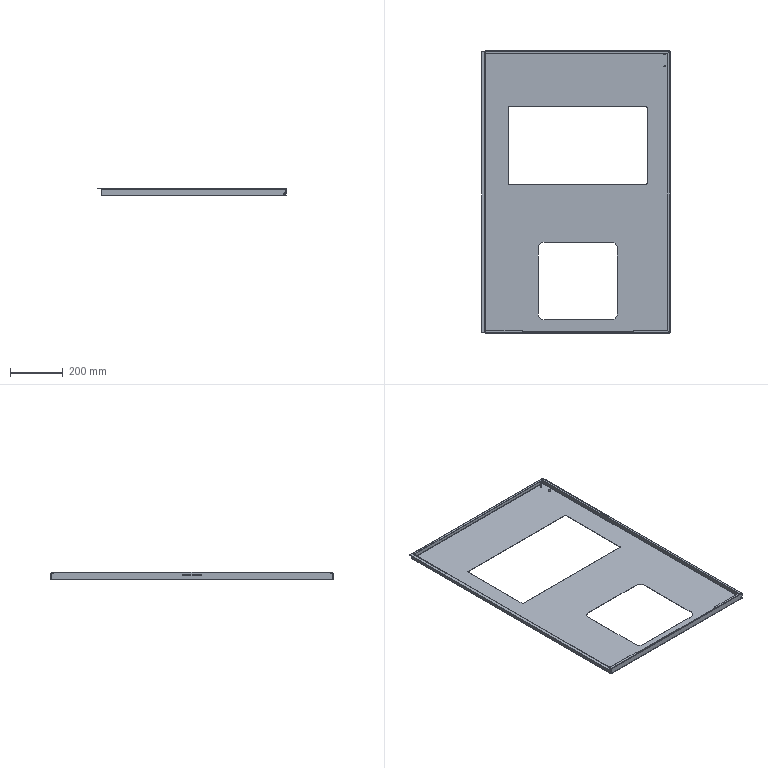Part | SolidWorks | features Fillet 4, Cut 3, EdgeFlange 3, ICE 3, FlatPattern 1, LPattern 1, SMBaseFlange 1, SheetMetal 1 | 1 solid | 108 faces | box 713.5 x 1066 x 27.237 mm | volume 927429 mm3 | plane 60 | cylinder 36 | spline 12 | commonest cylinder face diameters 1.473 x8 4.473 x8 5 x4 6.3 x4 8 x4 44 x4